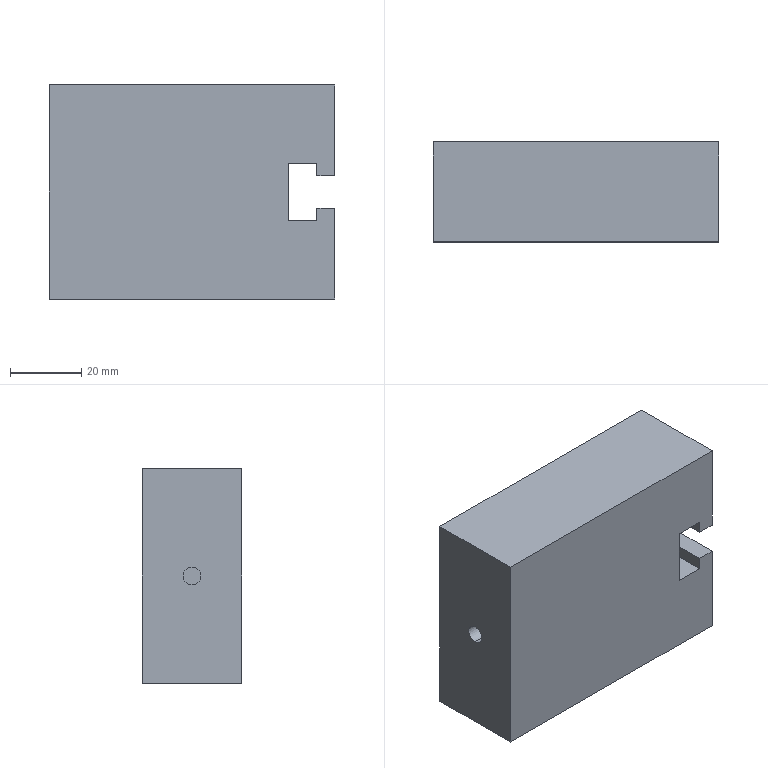Part | STEP file | 1 solid | 17 faces | box 80 x 28 x 60 mm | volume 129360 mm3 | plane 15 | cylinder 2 | commonest cylinder face diameters 5 x2
STEP:
#1=CARTESIAN_POINT('',(0.,0.,0.));
#2=DIRECTION('',(0.,0.,1.));
#3=DIRECTION('',(1.,0.,0.));
#4=AXIS2_PLACEMENT_3D('',#1,#2,#3);
#5=CARTESIAN_POINT('',(-30.,14.,2.5));
#6=VERTEX_POINT('',#5);
#7=CARTESIAN_POINT('',(-40.,14.,2.5));
#8=VERTEX_POINT('',#7);
#9=CARTESIAN_POINT('',(-30.,14.,2.5));
#10=DIRECTION('',(-1.,0.,0.));
#11=VECTOR('',#10,1.);
#12=LINE('',#9,#11);
#13=CARTESIAN_POINT('',(-30.,14.,0.));
#14=DIRECTION('',(-1.,0.,0.));
#15=DIRECTION('',(0.,0.,1.));
#16=AXIS2_PLACEMENT_3D('',#13,#14,#15);
#17=CYLINDRICAL_SURFACE('',#16,2.5);
#18=CARTESIAN_POINT('',(6.283,0.));
#19=DIRECTION('',(0.,1.));
#20=VECTOR('',#19,1.);
#21=LINE('',#18,#20);
#22=(GEOMETRIC_REPRESENTATION_CONTEXT(2)PARAMETRIC_REPRESENTATION_CONTEXT()REPRESENTATION_CONTEXT('',''));
#23=DEFINITIONAL_REPRESENTATION('',(#21),#22);
#24=PCURVE('',#17,#23);
#25=CARTESIAN_POINT('',(-30.,14.,0.));
#26=DIRECTION('',(-1.,0.,0.));
#27=DIRECTION('',(0.,0.,1.));
#28=AXIS2_PLACEMENT_3D('',#25,#26,#27);
#29=CYLINDRICAL_SURFACE('',#28,2.5);
#30=CARTESIAN_POINT('',(0.,0.));
#31=DIRECTION('',(0.,1.));
#32=VECTOR('',#31,1.);
#33=LINE('',#30,#32);
#34=(GEOMETRIC_REPRESENTATION_CONTEXT(2)PARAMETRIC_REPRESENTATION_CONTEXT()REPRESENTATION_CONTEXT('',''));
#35=DEFINITIONAL_REPRESENTATION('',(#33),#34);
#36=PCURVE('',#29,#35);
#37=SURFACE_CURVE('',#12,(#24,#36),.PCURVE_S1.);
#38=EDGE_CURVE('',#6,#8,#37,.T.);
#39=ORIENTED_EDGE('',*,*,#38,.T.);
#40=CARTESIAN_POINT('',(-40.,14.,-2.5));
#41=VERTEX_POINT('',#40);
#42=CARTESIAN_POINT('',(-40.,14.,0.));
#43=DIRECTION('',(-1.,0.,0.));
#44=DIRECTION('',(0.,0.,1.));
#45=AXIS2_PLACEMENT_3D('',#42,#43,#44);
#46=CIRCLE('',#45,2.5);
#47=CARTESIAN_POINT('',(0.,10.));
#48=DIRECTION('',(1.,0.));
#49=VECTOR('',#48,1.);
#50=LINE('',#47,#49);
#51=(GEOMETRIC_REPRESENTATION_CONTEXT(2)PARAMETRIC_REPRESENTATION_CONTEXT()REPRESENTATION_CONTEXT('',''));
#52=DEFINITIONAL_REPRESENTATION('',(#50),#51);
#53=PCURVE('',#17,#52);
#54=CARTESIAN_POINT('',(-40.,28.,30.));
#55=DIRECTION('',(1.,0.,0.));
#56=DIRECTION('',(0.,0.,-1.));
#57=AXIS2_PLACEMENT_3D('',#54,#55,#56);
#58=PLANE('',#57);
#59=CARTESIAN_POINT('',(27.5,-14.));
#60=CARTESIAN_POINT('',(27.5,-9.67));
#61=CARTESIAN_POINT('',(31.25,-11.835));
#62=CARTESIAN_POINT('',(35.,-14.));
#63=CARTESIAN_POINT('',(31.25,-16.165));
#64=CARTESIAN_POINT('',(27.5,-18.33));
#65=CARTESIAN_POINT('',(27.5,-14.));
#66=(BOUNDED_CURVE()B_SPLINE_CURVE(2,(#59,#60,#61,#62,#63,#64,#65),.UNSPECIFIED.,.T.,.F.)B_SPLINE_CURVE_WITH_KNOTS((1,2,2,2,2,1),(-2.094,0.,2.094,4.189,6.283,8.378),.UNSPECIFIED.)CURVE()GEOMETRIC_REPRESENTATION_ITEM()RATIONAL_B_SPLINE_CURVE((1.,0.5,1.,0.5,1.,0.5,1.))REPRESENTATION_ITEM(''));
#67=(GEOMETRIC_REPRESENTATION_CONTEXT(2)PARAMETRIC_REPRESENTATION_CONTEXT()REPRESENTATION_CONTEXT('',''));
#68=DEFINITIONAL_REPRESENTATION('',(#66),#67);
#69=PCURVE('',#58,#68);
#70=SURFACE_CURVE('',#46,(#53,#69),.PCURVE_S1.);
#71=EDGE_CURVE('',#41,#8,#70,.T.);
#72=ORIENTED_EDGE('',*,*,#71,.F.);
#73=CARTESIAN_POINT('',(-30.,14.,-2.5));
#74=VERTEX_POINT('',#73);
#75=CARTESIAN_POINT('',(-30.,14.,-2.5));
#76=DIRECTION('',(-1.,0.,0.));
#77=VECTOR('',#76,1.);
#78=LINE('',#75,#77);
#79=CARTESIAN_POINT('',(3.142,0.));
#80=DIRECTION('',(0.,1.));
#81=VECTOR('',#80,1.);
#82=LINE('',#79,#81);
#83=(GEOMETRIC_REPRESENTATION_CONTEXT(2)PARAMETRIC_REPRESENTATION_CONTEXT()REPRESENTATION_CONTEXT('',''));
#84=DEFINITIONAL_REPRESENTATION('',(#82),#83);
#85=PCURVE('',#17,#84);
#86=CARTESIAN_POINT('',(3.142,0.));
#87=DIRECTION('',(0.,1.));
#88=VECTOR('',#87,1.);
#89=LINE('',#86,#88);
#90=(GEOMETRIC_REPRESENTATION_CONTEXT(2)PARAMETRIC_REPRESENTATION_CONTEXT()REPRESENTATION_CONTEXT('',''));
#91=DEFINITIONAL_REPRESENTATION('',(#89),#90);
#92=PCURVE('',#29,#91);
#93=SURFACE_CURVE('',#78,(#85,#92),.PCURVE_S1.);
#94=EDGE_CURVE('',#74,#41,#93,.T.);
#95=ORIENTED_EDGE('',*,*,#94,.F.);
#96=CARTESIAN_POINT('',(-30.,14.,0.));
#97=DIRECTION('',(-1.,0.,0.));
#98=DIRECTION('',(0.,0.,1.));
#99=AXIS2_PLACEMENT_3D('',#96,#97,#98);
#100=CIRCLE('',#99,2.5);
#101=CARTESIAN_POINT('',(0.,0.));
#102=DIRECTION('',(1.,0.));
#103=VECTOR('',#102,1.);
#104=LINE('',#101,#103);
#105=(GEOMETRIC_REPRESENTATION_CONTEXT(2)PARAMETRIC_REPRESENTATION_CONTEXT()REPRESENTATION_CONTEXT('',''));
#106=DEFINITIONAL_REPRESENTATION('',(#104),#105);
#107=PCURVE('',#17,#106);
#108=CARTESIAN_POINT('',(-30.,14.,0.));
#109=DIRECTION('',(-1.,0.,0.));
#110=DIRECTION('',(0.,0.,1.));
#111=AXIS2_PLACEMENT_3D('',#108,#109,#110);
#112=PLANE('',#111);
#113=CARTESIAN_POINT('',(0.,0.));
#114=DIRECTION('',(1.,0.));
#115=AXIS2_PLACEMENT_2D('',#113,#114);
#116=CIRCLE('',#115,2.5);
#117=(GEOMETRIC_REPRESENTATION_CONTEXT(2)PARAMETRIC_REPRESENTATION_CONTEXT()REPRESENTATION_CONTEXT('',''));
#118=DEFINITIONAL_REPRESENTATION('',(#116),#117);
#119=PCURVE('',#112,#118);
#120=SURFACE_CURVE('',#100,(#107,#119),.PCURVE_S1.);
#121=EDGE_CURVE('',#74,#6,#120,.T.);
#122=ORIENTED_EDGE('',*,*,#121,.T.);
#123=EDGE_LOOP('',(#39,#72,#95,#122));
#124=FACE_BOUND('',#123,.F.);
#125=ADVANCED_FACE('',(#124),#17,.F.);
#126=CARTESIAN_POINT('',(40.,0.,30.));
#127=VERTEX_POINT('',#126);
#128=CARTESIAN_POINT('',(40.,0.,4.5));
#129=VERTEX_POINT('',#128);
#130=CARTESIAN_POINT('',(40.,0.,30.));
#131=DIRECTION('',(0.,0.,-1.));
#132=VECTOR('',#131,1.);
#133=LINE('',#130,#132);
#134=CARTESIAN_POINT('',(40.,28.,30.));
#135=DIRECTION('',(-1.,0.,0.));
#136=DIRECTION('',(0.,0.,1.));
#137=AXIS2_PLACEMENT_3D('',#134,#135,#136);
#138=PLANE('',#137);
#139=CARTESIAN_POINT('',(0.,-28.));
#140=DIRECTION('',(-1.,0.));
#141=VECTOR('',#140,1.);
#142=LINE('',#139,#141);
#143=(GEOMETRIC_REPRESENTATION_CONTEXT(2)PARAMETRIC_REPRESENTATION_CONTEXT()REPRESENTATION_CONTEXT('',''));
#144=DEFINITIONAL_REPRESENTATION('',(#142),#143);
#145=PCURVE('',#138,#144);
#146=CARTESIAN_POINT('',(0.,0.,0.));
#147=DIRECTION('',(0.,1.,0.));
#148=DIRECTION('',(0.,0.,1.));
#149=AXIS2_PLACEMENT_3D('',#146,#147,#148);
#150=PLANE('',#149);
#151=CARTESIAN_POINT('',(30.,40.));
#152=DIRECTION('',(-1.,0.));
#153=VECTOR('',#152,1.);
#154=LINE('',#151,#153);
#155=(GEOMETRIC_REPRESENTATION_CONTEXT(2)PARAMETRIC_REPRESENTATION_CONTEXT()REPRESENTATION_CONTEXT('',''));
#156=DEFINITIONAL_REPRESENTATION('',(#154),#155);
#157=PCURVE('',#150,#156);
#158=SURFACE_CURVE('',#133,(#145,#157),.PCURVE_S1.);
#159=EDGE_CURVE('',#127,#129,#158,.T.);
#160=ORIENTED_EDGE('',*,*,#159,.T.);
#161=CARTESIAN_POINT('',(40.,28.,4.5));
#162=VERTEX_POINT('',#161);
#163=CARTESIAN_POINT('',(40.,0.,4.5));
#164=DIRECTION('',(0.,1.,0.));
#165=VECTOR('',#164,1.);
#166=LINE('',#163,#165);
#167=CARTESIAN_POINT('',(-25.5,-28.));
#168=DIRECTION('',(0.,1.));
#169=VECTOR('',#168,1.);
#170=LINE('',#167,#169);
#171=(GEOMETRIC_REPRESENTATION_CONTEXT(2)PARAMETRIC_REPRESENTATION_CONTEXT()REPRESENTATION_CONTEXT('',''));
#172=DEFINITIONAL_REPRESENTATION('',(#170),#171);
#173=PCURVE('',#138,#172);
#174=CARTESIAN_POINT('',(40.,0.,4.5));
#175=DIRECTION('',(0.,0.,1.));
#176=DIRECTION('',(1.,0.,0.));
#177=AXIS2_PLACEMENT_3D('',#174,#175,#176);
#178=PLANE('',#177);
#179=CARTESIAN_POINT('',(0.,0.));
#180=DIRECTION('',(0.,1.));
#181=VECTOR('',#180,1.);
#182=LINE('',#179,#181);
#183=(GEOMETRIC_REPRESENTATION_CONTEXT(2)PARAMETRIC_REPRESENTATION_CONTEXT()REPRESENTATION_CONTEXT('',''));
#184=DEFINITIONAL_REPRESENTATION('',(#182),#183);
#185=PCURVE('',#178,#184);
#186=SURFACE_CURVE('',#166,(#173,#185),.PCURVE_S1.);
#187=EDGE_CURVE('',#129,#162,#186,.T.);
#188=ORIENTED_EDGE('',*,*,#187,.T.);
#189=CARTESIAN_POINT('',(40.,28.,30.));
#190=VERTEX_POINT('',#189);
#191=CARTESIAN_POINT('',(40.,28.,30.));
#192=DIRECTION('',(0.,0.,-1.));
#193=VECTOR('',#192,1.);
#194=LINE('',#191,#193);
#195=CARTESIAN_POINT('',(0.,0.));
#196=DIRECTION('',(-1.,0.));
#197=VECTOR('',#196,1.);
#198=LINE('',#195,#197);
#199=(GEOMETRIC_REPRESENTATION_CONTEXT(2)PARAMETRIC_REPRESENTATION_CONTEXT()REPRESENTATION_CONTEXT('',''));
#200=DEFINITIONAL_REPRESENTATION('',(#198),#199);
#201=PCURVE('',#138,#200);
#202=CARTESIAN_POINT('',(0.,28.,0.));
#203=DIRECTION('',(0.,1.,0.));
#204=DIRECTION('',(0.,0.,1.));
#205=AXIS2_PLACEMENT_3D('',#202,#203,#204);
#206=PLANE('',#205);
#207=CARTESIAN_POINT('',(30.,40.));
#208=DIRECTION('',(-1.,0.));
#209=VECTOR('',#208,1.);
#210=LINE('',#207,#209);
#211=(GEOMETRIC_REPRESENTATION_CONTEXT(2)PARAMETRIC_REPRESENTATION_CONTEXT()REPRESENTATION_CONTEXT('',''));
#212=DEFINITIONAL_REPRESENTATION('',(#210),#211);
#213=PCURVE('',#206,#212);
#214=SURFACE_CURVE('',#194,(#201,#213),.PCURVE_S1.);
#215=EDGE_CURVE('',#190,#162,#214,.T.);
#216=ORIENTED_EDGE('',*,*,#215,.F.);
#217=CARTESIAN_POINT('',(40.,28.,30.));
#218=DIRECTION('',(0.,-1.,0.));
#219=VECTOR('',#218,1.);
#220=LINE('',#217,#219);
#221=CARTESIAN_POINT('',(0.,0.));
#222=DIRECTION('',(0.,-1.));
#223=VECTOR('',#222,1.);
#224=LINE('',#221,#223);
#225=(GEOMETRIC_REPRESENTATION_CONTEXT(2)PARAMETRIC_REPRESENTATION_CONTEXT()REPRESENTATION_CONTEXT('',''));
#226=DEFINITIONAL_REPRESENTATION('',(#224),#225);
#227=PCURVE('',#138,#226);
#228=CARTESIAN_POINT('',(40.,28.,30.));
#229=DIRECTION('',(0.,0.,-1.));
#230=DIRECTION('',(-1.,0.,0.));
#231=AXIS2_PLACEMENT_3D('',#228,#229,#230);
#232=PLANE('',#231);
#233=CARTESIAN_POINT('',(0.,0.));
#234=DIRECTION('',(0.,-1.));
#235=VECTOR('',#234,1.);
#236=LINE('',#233,#235);
#237=(GEOMETRIC_REPRESENTATION_CONTEXT(2)PARAMETRIC_REPRESENTATION_CONTEXT()REPRESENTATION_CONTEXT('',''));
#238=DEFINITIONAL_REPRESENTATION('',(#236),#237);
#239=PCURVE('',#232,#238);
#240=SURFACE_CURVE('',#220,(#227,#239),.PCURVE_S1.);
#241=EDGE_CURVE('',#190,#127,#240,.T.);
#242=ORIENTED_EDGE('',*,*,#241,.T.);
#243=EDGE_LOOP('',(#160,#188,#216,#242));
#244=FACE_BOUND('',#243,.T.);
#245=ADVANCED_FACE('',(#244),#138,.F.);
#246=CARTESIAN_POINT('',(-40.,14.,0.));
#247=DIRECTION('',(-1.,0.,0.));
#248=DIRECTION('',(0.,0.,1.));
#249=AXIS2_PLACEMENT_3D('',#246,#247,#248);
#250=CIRCLE('',#249,2.5);
#251=CARTESIAN_POINT('',(27.5,-14.));
#252=CARTESIAN_POINT('',(27.5,-9.67));
#253=CARTESIAN_POINT('',(31.25,-11.835));
#254=CARTESIAN_POINT('',(35.,-14.));
#255=CARTESIAN_POINT('',(31.25,-16.165));
#256=CARTESIAN_POINT('',(27.5,-18.33));
#257=CARTESIAN_POINT('',(27.5,-14.));
#258=(BOUNDED_CURVE()B_SPLINE_CURVE(2,(#251,#252,#253,#254,#255,#256,#257),.UNSPECIFIED.,.T.,.F.)B_SPLINE_CURVE_WITH_KNOTS((1,2,2,2,2,1),(-2.094,0.,2.094,4.189,6.283,8.378),.UNSPECIFIED.)CURVE()GEOMETRIC_REPRESENTATION_ITEM()RATIONAL_B_SPLINE_CURVE((1.,0.5,1.,0.5,1.,0.5,1.))REPRESENTATION_ITEM(''));
#259=(GEOMETRIC_REPRESENTATION_CONTEXT(2)PARAMETRIC_REPRESENTATION_CONTEXT()REPRESENTATION_CONTEXT('',''));
#260=DEFINITIONAL_REPRESENTATION('',(#258),#259);
#261=PCURVE('',#58,#260);
#262=CARTESIAN_POINT('',(0.,10.));
#263=DIRECTION('',(1.,0.));
#264=VECTOR('',#263,1.);
#265=LINE('',#262,#264);
#266=(GEOMETRIC_REPRESENTATION_CONTEXT(2)PARAMETRIC_REPRESENTATION_CONTEXT()REPRESENTATION_CONTEXT('',''));
#267=DEFINITIONAL_REPRESENTATION('',(#265),#266);
#268=PCURVE('',#29,#267);
#269=SURFACE_CURVE('',#250,(#261,#268),.PCURVE_S1.);
#270=EDGE_CURVE('',#8,#41,#269,.T.);
#271=ORIENTED_EDGE('',*,*,#270,.F.);
#272=ORIENTED_EDGE('',*,*,#71,.F.);
#273=EDGE_LOOP('',(#271,#272));
#274=FACE_BOUND('',#273,.T.);
#275=CARTESIAN_POINT('',(-40.,0.,-30.));
#276=VERTEX_POINT('',#275);
#277=CARTESIAN_POINT('',(-40.,0.,30.));
#278=VERTEX_POINT('',#277);
#279=CARTESIAN_POINT('',(-40.,0.,30.));
#280=DIRECTION('',(0.,0.,1.));
#281=VECTOR('',#280,1.);
#282=LINE('',#279,#281);
#283=CARTESIAN_POINT('',(0.,-28.));
#284=DIRECTION('',(-1.,0.));
#285=VECTOR('',#284,1.);
#286=LINE('',#283,#285);
#287=(GEOMETRIC_REPRESENTATION_CONTEXT(2)PARAMETRIC_REPRESENTATION_CONTEXT()REPRESENTATION_CONTEXT('',''));
#288=DEFINITIONAL_REPRESENTATION('',(#286),#287);
#289=PCURVE('',#58,#288);
#290=CARTESIAN_POINT('',(30.,-40.));
#291=DIRECTION('',(1.,0.));
#292=VECTOR('',#291,1.);
#293=LINE('',#290,#292);
#294=(GEOMETRIC_REPRESENTATION_CONTEXT(2)PARAMETRIC_REPRESENTATION_CONTEXT()REPRESENTATION_CONTEXT('',''));
#295=DEFINITIONAL_REPRESENTATION('',(#293),#294);
#296=PCURVE('',#150,#295);
#297=SURFACE_CURVE('',#282,(#289,#296),.PCURVE_S1.);
#298=EDGE_CURVE('',#276,#278,#297,.T.);
#299=ORIENTED_EDGE('',*,*,#298,.T.);
#300=CARTESIAN_POINT('',(-40.,28.,30.));
#301=VERTEX_POINT('',#300);
#302=CARTESIAN_POINT('',(-40.,28.,30.));
#303=DIRECTION('',(0.,-1.,0.));
#304=VECTOR('',#303,1.);
#305=LINE('',#302,#304);
#306=CARTESIAN_POINT('',(0.,0.));
#307=DIRECTION('',(0.,-1.));
#308=VECTOR('',#307,1.);
#309=LINE('',#306,#308);
#310=(GEOMETRIC_REPRESENTATION_CONTEXT(2)PARAMETRIC_REPRESENTATION_CONTEXT()REPRESENTATION_CONTEXT('',''));
#311=DEFINITIONAL_REPRESENTATION('',(#309),#310);
#312=PCURVE('',#58,#311);
#313=CARTESIAN_POINT('',(80.,0.));
#314=DIRECTION('',(0.,-1.));
#315=VECTOR('',#314,1.);
#316=LINE('',#313,#315);
#317=(GEOMETRIC_REPRESENTATION_CONTEXT(2)PARAMETRIC_REPRESENTATION_CONTEXT()REPRESENTATION_CONTEXT('',''));
#318=DEFINITIONAL_REPRESENTATION('',(#316),#317);
#319=PCURVE('',#232,#318);
#320=SURFACE_CURVE('',#305,(#312,#319),.PCURVE_S1.);
#321=EDGE_CURVE('',#301,#278,#320,.T.);
#322=ORIENTED_EDGE('',*,*,#321,.F.);
#323=CARTESIAN_POINT('',(-40.,28.,-30.));
#324=VERTEX_POINT('',#323);
#325=CARTESIAN_POINT('',(-40.,28.,30.));
#326=DIRECTION('',(0.,0.,1.));
#327=VECTOR('',#326,1.);
#328=LINE('',#325,#327);
#329=CARTESIAN_POINT('',(0.,0.));
#330=DIRECTION('',(-1.,0.));
#331=VECTOR('',#330,1.);
#332=LINE('',#329,#331);
#333=(GEOMETRIC_REPRESENTATION_CONTEXT(2)PARAMETRIC_REPRESENTATION_CONTEXT()REPRESENTATION_CONTEXT('',''));
#334=DEFINITIONAL_REPRESENTATION('',(#332),#333);
#335=PCURVE('',#58,#334);
#336=CARTESIAN_POINT('',(30.,-40.));
#337=DIRECTION('',(1.,0.));
#338=VECTOR('',#337,1.);
#339=LINE('',#336,#338);
#340=(GEOMETRIC_REPRESENTATION_CONTEXT(2)PARAMETRIC_REPRESENTATION_CONTEXT()REPRESENTATION_CONTEXT('',''));
#341=DEFINITIONAL_REPRESENTATION('',(#339),#340);
#342=PCURVE('',#206,#341);
#343=SURFACE_CURVE('',#328,(#335,#342),.PCURVE_S1.);
#344=EDGE_CURVE('',#324,#301,#343,.T.);
#345=ORIENTED_EDGE('',*,*,#344,.F.);
#346=CARTESIAN_POINT('',(-40.,28.,-30.));
#347=DIRECTION('',(0.,-1.,0.));
#348=VECTOR('',#347,1.);
#349=LINE('',#346,#348);
#350=CARTESIAN_POINT('',(60.,0.));
#351=DIRECTION('',(0.,-1.));
#352=VECTOR('',#351,1.);
#353=LINE('',#350,#352);
#354=(GEOMETRIC_REPRESENTATION_CONTEXT(2)PARAMETRIC_REPRESENTATION_CONTEXT()REPRESENTATION_CONTEXT('',''));
#355=DEFINITIONAL_REPRESENTATION('',(#353),#354);
#356=PCURVE('',#58,#355);
#357=CARTESIAN_POINT('',(40.,28.,-30.));
#358=DIRECTION('',(0.,0.,1.));
#359=DIRECTION('',(1.,0.,0.));
#360=AXIS2_PLACEMENT_3D('',#357,#358,#359);
#361=PLANE('',#360);
#362=CARTESIAN_POINT('',(-80.,0.));
#363=DIRECTION('',(0.,-1.));
#364=VECTOR('',#363,1.);
#365=LINE('',#362,#364);
#366=(GEOMETRIC_REPRESENTATION_CONTEXT(2)PARAMETRIC_REPRESENTATION_CONTEXT()REPRESENTATION_CONTEXT('',''));
#367=DEFINITIONAL_REPRESENTATION('',(#365),#366);
#368=PCURVE('',#361,#367);
#369=SURFACE_CURVE('',#349,(#356,#368),.PCURVE_S1.);
#370=EDGE_CURVE('',#324,#276,#369,.T.);
#371=ORIENTED_EDGE('',*,*,#370,.T.);
#372=EDGE_LOOP('',(#299,#322,#345,#371));
#373=FACE_BOUND('',#372,.T.);
#374=ADVANCED_FACE('',(#274,#373),#58,.F.);
#375=CARTESIAN_POINT('',(40.,0.,30.));
#376=DIRECTION('',(1.,0.,0.));
#377=VECTOR('',#376,1.);
#378=LINE('',#375,#377);
#379=CARTESIAN_POINT('',(0.,-28.));
#380=DIRECTION('',(-1.,0.));
#381=VECTOR('',#380,1.);
#382=LINE('',#379,#381);
#383=(GEOMETRIC_REPRESENTATION_CONTEXT(2)PARAMETRIC_REPRESENTATION_CONTEXT()REPRESENTATION_CONTEXT('',''));
#384=DEFINITIONAL_REPRESENTATION('',(#382),#383);
#385=PCURVE('',#232,#384);
#386=CARTESIAN_POINT('',(30.,40.));
#387=DIRECTION('',(0.,1.));
#388=VECTOR('',#387,1.);
#389=LINE('',#386,#388);
#390=(GEOMETRIC_REPRESENTATION_CONTEXT(2)PARAMETRIC_REPRESENTATION_CONTEXT()REPRESENTATION_CONTEXT('',''));
#391=DEFINITIONAL_REPRESENTATION('',(#389),#390);
#392=PCURVE('',#150,#391);
#393=SURFACE_CURVE('',#378,(#385,#392),.PCURVE_S1.);
#394=EDGE_CURVE('',#278,#127,#393,.T.);
#395=ORIENTED_EDGE('',*,*,#394,.T.);
#396=ORIENTED_EDGE('',*,*,#241,.F.);
#397=CARTESIAN_POINT('',(40.,28.,30.));
#398=DIRECTION('',(1.,0.,0.));
#399=VECTOR('',#398,1.);
#400=LINE('',#397,#399);
#401=CARTESIAN_POINT('',(0.,0.));
#402=DIRECTION('',(-1.,0.));
#403=VECTOR('',#402,1.);
#404=LINE('',#401,#403);
#405=(GEOMETRIC_REPRESENTATION_CONTEXT(2)PARAMETRIC_REPRESENTATION_CONTEXT()REPRESENTATION_CONTEXT('',''));
#406=DEFINITIONAL_REPRESENTATION('',(#404),#405);
#407=PCURVE('',#232,#406);
#408=CARTESIAN_POINT('',(30.,40.));
#409=DIRECTION('',(0.,1.));
#410=VECTOR('',#409,1.);
#411=LINE('',#408,#410);
#412=(GEOMETRIC_REPRESENTATION_CONTEXT(2)PARAMETRIC_REPRESENTATION_CONTEXT()REPRESENTATION_CONTEXT('',''));
#413=DEFINITIONAL_REPRESENTATION('',(#411),#412);
#414=PCURVE('',#206,#413);
#415=SURFACE_CURVE('',#400,(#407,#414),.PCURVE_S1.);
#416=EDGE_CURVE('',#301,#190,#415,.T.);
#417=ORIENTED_EDGE('',*,*,#416,.F.);
#418=ORIENTED_EDGE('',*,*,#321,.T.);
#419=EDGE_LOOP('',(#395,#396,#417,#418));
#420=FACE_BOUND('',#419,.T.);
#421=ADVANCED_FACE('',(#420),#232,.F.);
#422=CARTESIAN_POINT('',(40.,28.,-4.5));
#423=VERTEX_POINT('',#422);
#424=CARTESIAN_POINT('',(40.,28.,-30.));
#425=VERTEX_POINT('',#424);
#426=CARTESIAN_POINT('',(40.,28.,30.));
#427=DIRECTION('',(0.,0.,-1.));
#428=VECTOR('',#427,1.);
#429=LINE('',#426,#428);
#430=CARTESIAN_POINT('',(40.,28.,30.));
#431=DIRECTION('',(-1.,0.,0.));
#432=DIRECTION('',(0.,0.,1.));
#433=AXIS2_PLACEMENT_3D('',#430,#431,#432);
#434=PLANE('',#433);
#435=CARTESIAN_POINT('',(0.,0.));
#436=DIRECTION('',(-1.,0.));
#437=VECTOR('',#436,1.);
#438=LINE('',#435,#437);
#439=(GEOMETRIC_REPRESENTATION_CONTEXT(2)PARAMETRIC_REPRESENTATION_CONTEXT()REPRESENTATION_CONTEXT('',''));
#440=DEFINITIONAL_REPRESENTATION('',(#438),#439);
#441=PCURVE('',#434,#440);
#442=CARTESIAN_POINT('',(30.,40.));
#443=DIRECTION('',(-1.,0.));
#444=VECTOR('',#443,1.);
#445=LINE('',#442,#444);
#446=(GEOMETRIC_REPRESENTATION_CONTEXT(2)PARAMETRIC_REPRESENTATION_CONTEXT()REPRESENTATION_CONTEXT('',''));
#447=DEFINITIONAL_REPRESENTATION('',(#445),#446);
#448=PCURVE('',#206,#447);
#449=SURFACE_CURVE('',#429,(#441,#448),.PCURVE_S1.);
#450=EDGE_CURVE('',#423,#425,#449,.T.);
#451=ORIENTED_EDGE('',*,*,#450,.F.);
#452=CARTESIAN_POINT('',(40.,0.,-4.5));
#453=VERTEX_POINT('',#452);
#454=CARTESIAN_POINT('',(40.,0.,-4.5));
#455=DIRECTION('',(0.,1.,0.));
#456=VECTOR('',#455,1.);
#457=LINE('',#454,#456);
#458=CARTESIAN_POINT('',(-34.5,-28.));
#459=DIRECTION('',(0.,1.));
#460=VECTOR('',#459,1.);
#461=LINE('',#458,#460);
#462=(GEOMETRIC_REPRESENTATION_CONTEXT(2)PARAMETRIC_REPRESENTATION_CONTEXT()REPRESENTATION_CONTEXT('',''));
#463=DEFINITIONAL_REPRESENTATION('',(#461),#462);
#464=PCURVE('',#434,#463);
#465=CARTESIAN_POINT('',(40.,0.,-4.5));
#466=DIRECTION('',(0.,0.,-1.));
#467=DIRECTION('',(-1.,0.,0.));
#468=AXIS2_PLACEMENT_3D('',#465,#466,#467);
#469=PLANE('',#468);
#470=CARTESIAN_POINT('',(0.,0.));
#471=DIRECTION('',(0.,1.));
#472=VECTOR('',#471,1.);
#473=LINE('',#470,#472);
#474=(GEOMETRIC_REPRESENTATION_CONTEXT(2)PARAMETRIC_REPRESENTATION_CONTEXT()REPRESENTATION_CONTEXT('',''));
#475=DEFINITIONAL_REPRESENTATION('',(#473),#474);
#476=PCURVE('',#469,#475);
#477=SURFACE_CURVE('',#457,(#464,#476),.PCURVE_S1.);
#478=EDGE_CURVE('',#453,#423,#477,.T.);
#479=ORIENTED_EDGE('',*,*,#478,.F.);
#480=CARTESIAN_POINT('',(40.,0.,-30.));
#481=VERTEX_POINT('',#480);
#482=CARTESIAN_POINT('',(40.,0.,30.));
#483=DIRECTION('',(0.,0.,-1.));
#484=VECTOR('',#483,1.);
#485=LINE('',#482,#484);
#486=CARTESIAN_POINT('',(0.,-28.));
#487=DIRECTION('',(-1.,0.));
#488=VECTOR('',#487,1.);
#489=LINE('',#486,#488);
#490=(GEOMETRIC_REPRESENTATION_CONTEXT(2)PARAMETRIC_REPRESENTATION_CONTEXT()REPRESENTATION_CONTEXT('',''));
#491=DEFINITIONAL_REPRESENTATION('',(#489),#490);
#492=PCURVE('',#434,#491);
#493=CARTESIAN_POINT('',(30.,40.));
#494=DIRECTION('',(-1.,0.));
#495=VECTOR('',#494,1.);
#496=LINE('',#493,#495);
#497=(GEOMETRIC_REPRESENTATION_CONTEXT(2)PARAMETRIC_REPRESENTATION_CONTEXT()REPRESENTATION_CONTEXT('',''));
#498=DEFINITIONAL_REPRESENTATION('',(#496),#497);
#499=PCURVE('',#150,#498);
#500=SURFACE_CURVE('',#485,(#492,#499),.PCURVE_S1.);
#501=EDGE_CURVE('',#453,#481,#500,.T.);
#502=ORIENTED_EDGE('',*,*,#501,.T.);
#503=CARTESIAN_POINT('',(40.,28.,-30.));
#504=DIRECTION('',(0.,-1.,0.));
#505=VECTOR('',#504,1.);
#506=LINE('',#503,#505);
#507=CARTESIAN_POINT('',(-60.,0.));
#508=DIRECTION('',(0.,-1.));
#509=VECTOR('',#508,1.);
#510=LINE('',#507,#509);
#511=(GEOMETRIC_REPRESENTATION_CONTEXT(2)PARAMETRIC_REPRESENTATION_CONTEXT()REPRESENTATION_CONTEXT('',''));
#512=DEFINITIONAL_REPRESENTATION('',(#510),#511);
#513=PCURVE('',#434,#512);
#514=CARTESIAN_POINT('',(0.,0.));
#515=DIRECTION('',(0.,-1.));
#516=VECTOR('',#515,1.);
#517=LINE('',#514,#516);
#518=(GEOMETRIC_REPRESENTATION_CONTEXT(2)PARAMETRIC_REPRESENTATION_CONTEXT()REPRESENTATION_CONTEXT('',''));
#519=DEFINITIONAL_REPRESENTATION('',(#517),#518);
#520=PCURVE('',#361,#519);
#521=SURFACE_CURVE('',#506,(#513,#520),.PCURVE_S1.);
#522=EDGE_CURVE('',#425,#481,#521,.T.);
#523=ORIENTED_EDGE('',*,*,#522,.F.);
#524=EDGE_LOOP('',(#451,#479,#502,#523));
#525=FACE_BOUND('',#524,.T.);
#526=ADVANCED_FACE('',(#525),#434,.F.);
#527=CARTESIAN_POINT('',(40.,0.,-30.));
#528=DIRECTION('',(-1.,0.,0.));
#529=VECTOR('',#528,1.);
#530=LINE('',#527,#529);
#531=CARTESIAN_POINT('',(0.,-28.));
#532=DIRECTION('',(-1.,0.));
#533=VECTOR('',#532,1.);
#534=LINE('',#531,#533);
#535=(GEOMETRIC_REPRESENTATION_CONTEXT(2)PARAMETRIC_REPRESENTATION_CONTEXT()REPRESENTATION_CONTEXT('',''));
#536=DEFINITIONAL_REPRESENTATION('',(#534),#535);
#537=PCURVE('',#361,#536);
#538=CARTESIAN_POINT('',(-30.,40.));
#539=DIRECTION('',(0.,-1.));
#540=VECTOR('',#539,1.);
#541=LINE('',#538,#540);
#542=(GEOMETRIC_REPRESENTATION_CONTEXT(2)PARAMETRIC_REPRESENTATION_CONTEXT()REPRESENTATION_CONTEXT('',''));
#543=DEFINITIONAL_REPRESENTATION('',(#541),#542);
#544=PCURVE('',#150,#543);
#545=SURFACE_CURVE('',#530,(#537,#544),.PCURVE_S1.);
#546=EDGE_CURVE('',#481,#276,#545,.T.);
#547=ORIENTED_EDGE('',*,*,#546,.T.);
#548=ORIENTED_EDGE('',*,*,#370,.F.);
#549=CARTESIAN_POINT('',(40.,28.,-30.));
#550=DIRECTION('',(-1.,0.,0.));
#551=VECTOR('',#550,1.);
#552=LINE('',#549,#551);
#553=CARTESIAN_POINT('',(0.,0.));
#554=DIRECTION('',(-1.,0.));
#555=VECTOR('',#554,1.);
#556=LINE('',#553,#555);
#557=(GEOMETRIC_REPRESENTATION_CONTEXT(2)PARAMETRIC_REPRESENTATION_CONTEXT()REPRESENTATION_CONTEXT('',''));
#558=DEFINITIONAL_REPRESENTATION('',(#556),#557);
#559=PCURVE('',#361,#558);
#560=CARTESIAN_POINT('',(-30.,40.));
#561=DIRECTION('',(0.,-1.));
#562=VECTOR('',#561,1.);
#563=LINE('',#560,#562);
#564=(GEOMETRIC_REPRESENTATION_CONTEXT(2)PARAMETRIC_REPRESENTATION_CONTEXT()REPRESENTATION_CONTEXT('',''));
#565=DEFINITIONAL_REPRESENTATION('',(#563),#564);
#566=PCURVE('',#206,#565);
#567=SURFACE_CURVE('',#552,(#559,#566),.PCURVE_S1.);
#568=EDGE_CURVE('',#425,#324,#567,.T.);
#569=ORIENTED_EDGE('',*,*,#568,.F.);
#570=ORIENTED_EDGE('',*,*,#522,.T.);
#571=EDGE_LOOP('',(#547,#548,#569,#570));
#572=FACE_BOUND('',#571,.T.);
#573=ADVANCED_FACE('',(#572),#361,.F.);
#574=CARTESIAN_POINT('',(35.,28.,4.5));
#575=VERTEX_POINT('',#574);
#576=CARTESIAN_POINT('',(40.,28.,4.5));
#577=DIRECTION('',(1.,0.,0.));
#578=VECTOR('',#577,1.);
#579=LINE('',#576,#578);
#580=CARTESIAN_POINT('',(4.5,40.));
#581=DIRECTION('',(0.,1.));
#582=VECTOR('',#581,1.);
#583=LINE('',#580,#582);
#584=(GEOMETRIC_REPRESENTATION_CONTEXT(2)PARAMETRIC_REPRESENTATION_CONTEXT()REPRESENTATION_CONTEXT('',''));
#585=DEFINITIONAL_REPRESENTATION('',(#583),#584);
#586=PCURVE('',#206,#585);
#587=CARTESIAN_POINT('',(0.,28.));
#588=DIRECTION('',(1.,0.));
#589=VECTOR('',#588,1.);
#590=LINE('',#587,#589);
#591=(GEOMETRIC_REPRESENTATION_CONTEXT(2)PARAMETRIC_REPRESENTATION_CONTEXT()REPRESENTATION_CONTEXT('',''));
#592=DEFINITIONAL_REPRESENTATION('',(#590),#591);
#593=PCURVE('',#178,#592);
#594=SURFACE_CURVE('',#579,(#586,#593),.PCURVE_S1.);
#595=EDGE_CURVE('',#575,#162,#594,.T.);
#596=ORIENTED_EDGE('',*,*,#595,.F.);
#597=CARTESIAN_POINT('',(35.,28.,8.));
#598=VERTEX_POINT('',#597);
#599=CARTESIAN_POINT('',(35.,28.,4.5));
#600=DIRECTION('',(0.,0.,-1.));
#601=VECTOR('',#600,1.);
#602=LINE('',#599,#601);
#603=CARTESIAN_POINT('',(4.5,35.));
#604=DIRECTION('',(-1.,0.));
#605=VECTOR('',#604,1.);
#606=LINE('',#603,#605);
#607=(GEOMETRIC_REPRESENTATION_CONTEXT(2)PARAMETRIC_REPRESENTATION_CONTEXT()REPRESENTATION_CONTEXT('',''));
#608=DEFINITIONAL_REPRESENTATION('',(#606),#607);
#609=PCURVE('',#206,#608);
#610=CARTESIAN_POINT('',(35.,0.,4.5));
#611=DIRECTION('',(1.,0.,0.));
#612=DIRECTION('',(0.,0.,-1.));
#613=AXIS2_PLACEMENT_3D('',#610,#611,#612);
#614=PLANE('',#613);
#615=CARTESIAN_POINT('',(0.,28.));
#616=DIRECTION('',(1.,0.));
#617=VECTOR('',#616,1.);
#618=LINE('',#615,#617);
#619=(GEOMETRIC_REPRESENTATION_CONTEXT(2)PARAMETRIC_REPRESENTATION_CONTEXT()REPRESENTATION_CONTEXT('',''));
#620=DEFINITIONAL_REPRESENTATION('',(#618),#619);
#621=PCURVE('',#614,#620);
#622=SURFACE_CURVE('',#602,(#609,#621),.PCURVE_S1.);
#623=EDGE_CURVE('',#598,#575,#622,.T.);
#624=ORIENTED_EDGE('',*,*,#623,.F.);
#625=CARTESIAN_POINT('',(27.,28.,8.));
#626=VERTEX_POINT('',#625);
#627=CARTESIAN_POINT('',(35.,28.,8.));
#628=DIRECTION('',(1.,0.,0.));
#629=VECTOR('',#628,1.);
#630=LINE('',#627,#629);
#631=CARTESIAN_POINT('',(8.,35.));
#632=DIRECTION('',(0.,1.));
#633=VECTOR('',#632,1.);
#634=LINE('',#631,#633);
#635=(GEOMETRIC_REPRESENTATION_CONTEXT(2)PARAMETRIC_REPRESENTATION_CONTEXT()REPRESENTATION_CONTEXT('',''));
#636=DEFINITIONAL_REPRESENTATION('',(#634),#635);
#637=PCURVE('',#206,#636);
#638=CARTESIAN_POINT('',(35.,0.,8.));
#639=DIRECTION('',(0.,0.,1.));
#640=DIRECTION('',(1.,0.,0.));
#641=AXIS2_PLACEMENT_3D('',#638,#639,#640);
#642=PLANE('',#641);
#643=CARTESIAN_POINT('',(0.,28.));
#644=DIRECTION('',(1.,0.));
#645=VECTOR('',#644,1.);
#646=LINE('',#643,#645);
#647=(GEOMETRIC_REPRESENTATION_CONTEXT(2)PARAMETRIC_REPRESENTATION_CONTEXT()REPRESENTATION_CONTEXT('',''));
#648=DEFINITIONAL_REPRESENTATION('',(#646),#647);
#649=PCURVE('',#642,#648);
#650=SURFACE_CURVE('',#630,(#637,#649),.PCURVE_S1.);
#651=EDGE_CURVE('',#626,#598,#650,.T.);
#652=ORIENTED_EDGE('',*,*,#651,.F.);
#653=CARTESIAN_POINT('',(27.,28.,-8.));
#654=VERTEX_POINT('',#653);
#655=CARTESIAN_POINT('',(27.,28.,-8.));
#656=DIRECTION('',(0.,0.,1.));
#657=VECTOR('',#656,1.);
#658=LINE('',#655,#657);
#659=CARTESIAN_POINT('',(-8.,27.));
#660=DIRECTION('',(1.,0.));
#661=VECTOR('',#660,1.);
#662=LINE('',#659,#661);
#663=(GEOMETRIC_REPRESENTATION_CONTEXT(2)PARAMETRIC_REPRESENTATION_CONTEXT()REPRESENTATION_CONTEXT('',''));
#664=DEFINITIONAL_REPRESENTATION('',(#662),#663);
#665=PCURVE('',#206,#664);
#666=CARTESIAN_POINT('',(27.,0.,-8.));
#667=DIRECTION('',(-1.,0.,0.));
#668=DIRECTION('',(0.,0.,1.));
#669=AXIS2_PLACEMENT_3D('',#666,#667,#668);
#670=PLANE('',#669);
#671=CARTESIAN_POINT('',(0.,28.));
#672=DIRECTION('',(1.,0.));
#673=VECTOR('',#672,1.);
#674=LINE('',#671,#673);
#675=(GEOMETRIC_REPRESENTATION_CONTEXT(2)PARAMETRIC_REPRESENTATION_CONTEXT()REPRESENTATION_CONTEXT('',''));
#676=DEFINITIONAL_REPRESENTATION('',(#674),#675);
#677=PCURVE('',#670,#676);
#678=SURFACE_CURVE('',#658,(#665,#677),.PCURVE_S1.);
#679=EDGE_CURVE('',#654,#626,#678,.T.);
#680=ORIENTED_EDGE('',*,*,#679,.F.);
#681=CARTESIAN_POINT('',(35.,28.,-8.));
#682=VERTEX_POINT('',#681);
#683=CARTESIAN_POINT('',(35.,28.,-8.));
#684=DIRECTION('',(-1.,0.,0.));
#685=VECTOR('',#684,1.);
#686=LINE('',#683,#685);
#687=CARTESIAN_POINT('',(-8.,35.));
#688=DIRECTION('',(0.,-1.));
#689=VECTOR('',#688,1.);
#690=LINE('',#687,#689);
#691=(GEOMETRIC_REPRESENTATION_CONTEXT(2)PARAMETRIC_REPRESENTATION_CONTEXT()REPRESENTATION_CONTEXT('',''));
#692=DEFINITIONAL_REPRESENTATION('',(#690),#691);
#693=PCURVE('',#206,#692);
#694=CARTESIAN_POINT('',(35.,0.,-8.));
#695=DIRECTION('',(0.,0.,-1.));
#696=DIRECTION('',(-1.,0.,0.));
#697=AXIS2_PLACEMENT_3D('',#694,#695,#696);
#698=PLANE('',#697);
#699=CARTESIAN_POINT('',(0.,28.));
#700=DIRECTION('',(1.,0.));
#701=VECTOR('',#700,1.);
#702=LINE('',#699,#701);
#703=(GEOMETRIC_REPRESENTATION_CONTEXT(2)PARAMETRIC_REPRESENTATION_CONTEXT()REPRESENTATION_CONTEXT('',''));
#704=DEFINITIONAL_REPRESENTATION('',(#702),#703);
#705=PCURVE('',#698,#704);
#706=SURFACE_CURVE('',#686,(#693,#705),.PCURVE_S1.);
#707=EDGE_CURVE('',#682,#654,#706,.T.);
#708=ORIENTED_EDGE('',*,*,#707,.F.);
#709=CARTESIAN_POINT('',(35.,28.,-4.5));
#710=VERTEX_POINT('',#709);
#711=CARTESIAN_POINT('',(35.,28.,-4.5));
#712=DIRECTION('',(0.,0.,-1.));
#713=VECTOR('',#712,1.);
#714=LINE('',#711,#713);
#715=CARTESIAN_POINT('',(-4.5,35.));
#716=DIRECTION('',(-1.,0.));
#717=VECTOR('',#716,1.);
#718=LINE('',#715,#717);
#719=(GEOMETRIC_REPRESENTATION_CONTEXT(2)PARAMETRIC_REPRESENTATION_CONTEXT()REPRESENTATION_CONTEXT('',''));
#720=DEFINITIONAL_REPRESENTATION('',(#718),#719);
#721=PCURVE('',#206,#720);
#722=CARTESIAN_POINT('',(35.,0.,-4.5));
#723=DIRECTION('',(1.,0.,0.));
#724=DIRECTION('',(0.,0.,-1.));
#725=AXIS2_PLACEMENT_3D('',#722,#723,#724);
#726=PLANE('',#725);
#727=CARTESIAN_POINT('',(0.,28.));
#728=DIRECTION('',(1.,0.));
#729=VECTOR('',#728,1.);
#730=LINE('',#727,#729);
#731=(GEOMETRIC_REPRESENTATION_CONTEXT(2)PARAMETRIC_REPRESENTATION_CONTEXT()REPRESENTATION_CONTEXT('',''));
#732=DEFINITIONAL_REPRESENTATION('',(#730),#731);
#733=PCURVE('',#726,#732);
#734=SURFACE_CURVE('',#714,(#721,#733),.PCURVE_S1.);
#735=EDGE_CURVE('',#710,#682,#734,.T.);
#736=ORIENTED_EDGE('',*,*,#735,.F.);
#737=CARTESIAN_POINT('',(40.,28.,-4.5));
#738=DIRECTION('',(-1.,0.,0.));
#739=VECTOR('',#738,1.);
#740=LINE('',#737,#739);
#741=CARTESIAN_POINT('',(-4.5,40.));
#742=DIRECTION('',(0.,-1.));
#743=VECTOR('',#742,1.);
#744=LINE('',#741,#743);
#745=(GEOMETRIC_REPRESENTATION_CONTEXT(2)PARAMETRIC_REPRESENTATION_CONTEXT()REPRESENTATION_CONTEXT('',''));
#746=DEFINITIONAL_REPRESENTATION('',(#744),#745);
#747=PCURVE('',#206,#746);
#748=CARTESIAN_POINT('',(0.,28.));
#749=DIRECTION('',(1.,0.));
#750=VECTOR('',#749,1.);
#751=LINE('',#748,#750);
#752=(GEOMETRIC_REPRESENTATION_CONTEXT(2)PARAMETRIC_REPRESENTATION_CONTEXT()REPRESENTATION_CONTEXT('',''));
#753=DEFINITIONAL_REPRESENTATION('',(#751),#752);
#754=PCURVE('',#469,#753);
#755=SURFACE_CURVE('',#740,(#747,#754),.PCURVE_S1.);
#756=EDGE_CURVE('',#423,#710,#755,.T.);
#757=ORIENTED_EDGE('',*,*,#756,.F.);
#758=ORIENTED_EDGE('',*,*,#450,.T.);
#759=ORIENTED_EDGE('',*,*,#568,.T.);
#760=ORIENTED_EDGE('',*,*,#344,.T.);
#761=ORIENTED_EDGE('',*,*,#416,.T.);
#762=ORIENTED_EDGE('',*,*,#215,.T.);
#763=EDGE_LOOP('',(#596,#624,#652,#680,#708,#736,#757,#758,#759,#760,#761,#762));
#764=FACE_BOUND('',#763,.T.);
#765=ADVANCED_FACE('',(#764),#206,.T.);
#766=CARTESIAN_POINT('',(35.,0.,8.));
#767=VERTEX_POINT('',#766);
#768=CARTESIAN_POINT('',(35.,0.,4.5));
#769=VERTEX_POINT('',#768);
#770=CARTESIAN_POINT('',(35.,0.,4.5));
#771=DIRECTION('',(0.,0.,-1.));
#772=VECTOR('',#771,1.);
#773=LINE('',#770,#772);
#774=CARTESIAN_POINT('',(4.5,35.));
#775=DIRECTION('',(-1.,0.));
#776=VECTOR('',#775,1.);
#777=LINE('',#774,#776);
#778=(GEOMETRIC_REPRESENTATION_CONTEXT(2)PARAMETRIC_REPRESENTATION_CONTEXT()REPRESENTATION_CONTEXT('',''));
#779=DEFINITIONAL_REPRESENTATION('',(#777),#778);
#780=PCURVE('',#150,#779);
#781=CARTESIAN_POINT('',(0.,0.));
#782=DIRECTION('',(1.,0.));
#783=VECTOR('',#782,1.);
#784=LINE('',#781,#783);
#785=(GEOMETRIC_REPRESENTATION_CONTEXT(2)PARAMETRIC_REPRESENTATION_CONTEXT()REPRESENTATION_CONTEXT('',''));
#786=DEFINITIONAL_REPRESENTATION('',(#784),#785);
#787=PCURVE('',#614,#786);
#788=SURFACE_CURVE('',#773,(#780,#787),.PCURVE_S1.);
#789=EDGE_CURVE('',#767,#769,#788,.T.);
#790=ORIENTED_EDGE('',*,*,#789,.T.);
#791=CARTESIAN_POINT('',(40.,0.,4.5));
#792=DIRECTION('',(1.,0.,0.));
#793=VECTOR('',#792,1.);
#794=LINE('',#791,#793);
#795=CARTESIAN_POINT('',(4.5,40.));
#796=DIRECTION('',(0.,1.));
#797=VECTOR('',#796,1.);
#798=LINE('',#795,#797);
#799=(GEOMETRIC_REPRESENTATION_CONTEXT(2)PARAMETRIC_REPRESENTATION_CONTEXT()REPRESENTATION_CONTEXT('',''));
#800=DEFINITIONAL_REPRESENTATION('',(#798),#799);
#801=PCURVE('',#150,#800);
#802=CARTESIAN_POINT('',(0.,0.));
#803=DIRECTION('',(1.,0.));
#804=VECTOR('',#803,1.);
#805=LINE('',#802,#804);
#806=(GEOMETRIC_REPRESENTATION_CONTEXT(2)PARAMETRIC_REPRESENTATION_CONTEXT()REPRESENTATION_CONTEXT('',''));
#807=DEFINITIONAL_REPRESENTATION('',(#805),#806);
#808=PCURVE('',#178,#807);
#809=SURFACE_CURVE('',#794,(#801,#808),.PCURVE_S1.);
#810=EDGE_CURVE('',#769,#129,#809,.T.);
#811=ORIENTED_EDGE('',*,*,#810,.T.);
#812=ORIENTED_EDGE('',*,*,#159,.F.);
#813=ORIENTED_EDGE('',*,*,#394,.F.);
#814=ORIENTED_EDGE('',*,*,#298,.F.);
#815=ORIENTED_EDGE('',*,*,#546,.F.);
#816=ORIENTED_EDGE('',*,*,#501,.F.);
#817=CARTESIAN_POINT('',(35.,0.,-4.5));
#818=VERTEX_POINT('',#817);
#819=CARTESIAN_POINT('',(40.,0.,-4.5));
#820=DIRECTION('',(-1.,0.,0.));
#821=VECTOR('',#820,1.);
#822=LINE('',#819,#821);
#823=CARTESIAN_POINT('',(-4.5,40.));
#824=DIRECTION('',(0.,-1.));
#825=VECTOR('',#824,1.);
#826=LINE('',#823,#825);
#827=(GEOMETRIC_REPRESENTATION_CONTEXT(2)PARAMETRIC_REPRESENTATION_CONTEXT()REPRESENTATION_CONTEXT('',''));
#828=DEFINITIONAL_REPRESENTATION('',(#826),#827);
#829=PCURVE('',#150,#828);
#830=CARTESIAN_POINT('',(0.,0.));
#831=DIRECTION('',(1.,0.));
#832=VECTOR('',#831,1.);
#833=LINE('',#830,#832);
#834=(GEOMETRIC_REPRESENTATION_CONTEXT(2)PARAMETRIC_REPRESENTATION_CONTEXT()REPRESENTATION_CONTEXT('',''));
#835=DEFINITIONAL_REPRESENTATION('',(#833),#834);
#836=PCURVE('',#469,#835);
#837=SURFACE_CURVE('',#822,(#829,#836),.PCURVE_S1.);
#838=EDGE_CURVE('',#453,#818,#837,.T.);
#839=ORIENTED_EDGE('',*,*,#838,.T.);
#840=CARTESIAN_POINT('',(35.,0.,-8.));
#841=VERTEX_POINT('',#840);
#842=CARTESIAN_POINT('',(35.,0.,-4.5));
#843=DIRECTION('',(0.,0.,-1.));
#844=VECTOR('',#843,1.);
#845=LINE('',#842,#844);
#846=CARTESIAN_POINT('',(-4.5,35.));
#847=DIRECTION('',(-1.,0.));
#848=VECTOR('',#847,1.);
#849=LINE('',#846,#848);
#850=(GEOMETRIC_REPRESENTATION_CONTEXT(2)PARAMETRIC_REPRESENTATION_CONTEXT()REPRESENTATION_CONTEXT('',''));
#851=DEFINITIONAL_REPRESENTATION('',(#849),#850);
#852=PCURVE('',#150,#851);
#853=CARTESIAN_POINT('',(0.,0.));
#854=DIRECTION('',(1.,0.));
#855=VECTOR('',#854,1.);
#856=LINE('',#853,#855);
#857=(GEOMETRIC_REPRESENTATION_CONTEXT(2)PARAMETRIC_REPRESENTATION_CONTEXT()REPRESENTATION_CONTEXT('',''));
#858=DEFINITIONAL_REPRESENTATION('',(#856),#857);
#859=PCURVE('',#726,#858);
#860=SURFACE_CURVE('',#845,(#852,#859),.PCURVE_S1.);
#861=EDGE_CURVE('',#818,#841,#860,.T.);
#862=ORIENTED_EDGE('',*,*,#861,.T.);
#863=CARTESIAN_POINT('',(27.,0.,-8.));
#864=VERTEX_POINT('',#863);
#865=CARTESIAN_POINT('',(35.,0.,-8.));
#866=DIRECTION('',(-1.,0.,0.));
#867=VECTOR('',#866,1.);
#868=LINE('',#865,#867);
#869=CARTESIAN_POINT('',(-8.,35.));
#870=DIRECTION('',(0.,-1.));
#871=VECTOR('',#870,1.);
#872=LINE('',#869,#871);
#873=(GEOMETRIC_REPRESENTATION_CONTEXT(2)PARAMETRIC_REPRESENTATION_CONTEXT()REPRESENTATION_CONTEXT('',''));
#874=DEFINITIONAL_REPRESENTATION('',(#872),#873);
#875=PCURVE('',#150,#874);
#876=CARTESIAN_POINT('',(0.,0.));
#877=DIRECTION('',(1.,0.));
#878=VECTOR('',#877,1.);
#879=LINE('',#876,#878);
#880=(GEOMETRIC_REPRESENTATION_CONTEXT(2)PARAMETRIC_REPRESENTATION_CONTEXT()REPRESENTATION_CONTEXT('',''));
#881=DEFINITIONAL_REPRESENTATION('',(#879),#880);
#882=PCURVE('',#698,#881);
#883=SURFACE_CURVE('',#868,(#875,#882),.PCURVE_S1.);
#884=EDGE_CURVE('',#841,#864,#883,.T.);
#885=ORIENTED_EDGE('',*,*,#884,.T.);
#886=CARTESIAN_POINT('',(27.,0.,8.));
#887=VERTEX_POINT('',#886);
#888=CARTESIAN_POINT('',(27.,0.,-8.));
#889=DIRECTION('',(0.,0.,1.));
#890=VECTOR('',#889,1.);
#891=LINE('',#888,#890);
#892=CARTESIAN_POINT('',(-8.,27.));
#893=DIRECTION('',(1.,0.));
#894=VECTOR('',#893,1.);
#895=LINE('',#892,#894);
#896=(GEOMETRIC_REPRESENTATION_CONTEXT(2)PARAMETRIC_REPRESENTATION_CONTEXT()REPRESENTATION_CONTEXT('',''));
#897=DEFINITIONAL_REPRESENTATION('',(#895),#896);
#898=PCURVE('',#150,#897);
#899=CARTESIAN_POINT('',(0.,0.));
#900=DIRECTION('',(1.,0.));
#901=VECTOR('',#900,1.);
#902=LINE('',#899,#901);
#903=(GEOMETRIC_REPRESENTATION_CONTEXT(2)PARAMETRIC_REPRESENTATION_CONTEXT()REPRESENTATION_CONTEXT('',''));
#904=DEFINITIONAL_REPRESENTATION('',(#902),#903);
#905=PCURVE('',#670,#904);
#906=SURFACE_CURVE('',#891,(#898,#905),.PCURVE_S1.);
#907=EDGE_CURVE('',#864,#887,#906,.T.);
#908=ORIENTED_EDGE('',*,*,#907,.T.);
#909=CARTESIAN_POINT('',(35.,0.,8.));
#910=DIRECTION('',(1.,0.,0.));
#911=VECTOR('',#910,1.);
#912=LINE('',#909,#911);
#913=CARTESIAN_POINT('',(8.,35.));
#914=DIRECTION('',(0.,1.));
#915=VECTOR('',#914,1.);
#916=LINE('',#913,#915);
#917=(GEOMETRIC_REPRESENTATION_CONTEXT(2)PARAMETRIC_REPRESENTATION_CONTEXT()REPRESENTATION_CONTEXT('',''));
#918=DEFINITIONAL_REPRESENTATION('',(#916),#917);
#919=PCURVE('',#150,#918);
#920=CARTESIAN_POINT('',(0.,0.));
#921=DIRECTION('',(1.,0.));
#922=VECTOR('',#921,1.);
#923=LINE('',#920,#922);
#924=(GEOMETRIC_REPRESENTATION_CONTEXT(2)PARAMETRIC_REPRESENTATION_CONTEXT()REPRESENTATION_CONTEXT('',''));
#925=DEFINITIONAL_REPRESENTATION('',(#923),#924);
#926=PCURVE('',#642,#925);
#927=SURFACE_CURVE('',#912,(#919,#926),.PCURVE_S1.);
#928=EDGE_CURVE('',#887,#767,#927,.T.);
#929=ORIENTED_EDGE('',*,*,#928,.T.);
#930=EDGE_LOOP('',(#790,#811,#812,#813,#814,#815,#816,#839,#862,#885,#908,#929));
#931=FACE_BOUND('',#930,.T.);
#932=ADVANCED_FACE('',(#931),#150,.F.);
#933=ORIENTED_EDGE('',*,*,#595,.T.);
#934=ORIENTED_EDGE('',*,*,#187,.F.);
#935=ORIENTED_EDGE('',*,*,#810,.F.);
#936=CARTESIAN_POINT('',(35.,0.,4.5));
#937=DIRECTION('',(0.,1.,0.));
#938=VECTOR('',#937,1.);
#939=LINE('',#936,#938);
#940=CARTESIAN_POINT('',(-5.,0.));
#941=DIRECTION('',(0.,1.));
#942=VECTOR('',#941,1.);
#943=LINE('',#940,#942);
#944=(GEOMETRIC_REPRESENTATION_CONTEXT(2)PARAMETRIC_REPRESENTATION_CONTEXT()REPRESENTATION_CONTEXT('',''));
#945=DEFINITIONAL_REPRESENTATION('',(#943),#944);
#946=PCURVE('',#178,#945);
#947=CARTESIAN_POINT('',(0.,0.));
#948=DIRECTION('',(0.,1.));
#949=VECTOR('',#948,1.);
#950=LINE('',#947,#949);
#951=(GEOMETRIC_REPRESENTATION_CONTEXT(2)PARAMETRIC_REPRESENTATION_CONTEXT()REPRESENTATION_CONTEXT('',''));
#952=DEFINITIONAL_REPRESENTATION('',(#950),#951);
#953=PCURVE('',#614,#952);
#954=SURFACE_CURVE('',#939,(#946,#953),.PCURVE_S1.);
#955=EDGE_CURVE('',#769,#575,#954,.T.);
#956=ORIENTED_EDGE('',*,*,#955,.T.);
#957=EDGE_LOOP('',(#933,#934,#935,#956));
#958=FACE_BOUND('',#957,.T.);
#959=ADVANCED_FACE('',(#958),#178,.F.);
#960=ORIENTED_EDGE('',*,*,#623,.T.);
#961=ORIENTED_EDGE('',*,*,#955,.F.);
#962=ORIENTED_EDGE('',*,*,#789,.F.);
#963=CARTESIAN_POINT('',(35.,0.,8.));
#964=DIRECTION('',(0.,1.,0.));
#965=VECTOR('',#964,1.);
#966=LINE('',#963,#965);
#967=CARTESIAN_POINT('',(-3.5,0.));
#968=DIRECTION('',(0.,1.));
#969=VECTOR('',#968,1.);
#970=LINE('',#967,#969);
#971=(GEOMETRIC_REPRESENTATION_CONTEXT(2)PARAMETRIC_REPRESENTATION_CONTEXT()REPRESENTATION_CONTEXT('',''));
#972=DEFINITIONAL_REPRESENTATION('',(#970),#971);
#973=PCURVE('',#614,#972);
#974=CARTESIAN_POINT('',(0.,0.));
#975=DIRECTION('',(0.,1.));
#976=VECTOR('',#975,1.);
#977=LINE('',#974,#976);
#978=(GEOMETRIC_REPRESENTATION_CONTEXT(2)PARAMETRIC_REPRESENTATION_CONTEXT()REPRESENTATION_CONTEXT('',''));
#979=DEFINITIONAL_REPRESENTATION('',(#977),#978);
#980=PCURVE('',#642,#979);
#981=SURFACE_CURVE('',#966,(#973,#980),.PCURVE_S1.);
#982=EDGE_CURVE('',#767,#598,#981,.T.);
#983=ORIENTED_EDGE('',*,*,#982,.T.);
#984=EDGE_LOOP('',(#960,#961,#962,#983));
#985=FACE_BOUND('',#984,.T.);
#986=ADVANCED_FACE('',(#985),#614,.F.);
#987=ORIENTED_EDGE('',*,*,#651,.T.);
#988=ORIENTED_EDGE('',*,*,#982,.F.);
#989=ORIENTED_EDGE('',*,*,#928,.F.);
#990=CARTESIAN_POINT('',(27.,0.,8.));
#991=DIRECTION('',(0.,1.,0.));
#992=VECTOR('',#991,1.);
#993=LINE('',#990,#992);
#994=CARTESIAN_POINT('',(-8.,0.));
#995=DIRECTION('',(0.,1.));
#996=VECTOR('',#995,1.);
#997=LINE('',#994,#996);
#998=(GEOMETRIC_REPRESENTATION_CONTEXT(2)PARAMETRIC_REPRESENTATION_CONTEXT()REPRESENTATION_CONTEXT('',''));
#999=DEFINITIONAL_REPRESENTATION('',(#997),#998);
#1000=PCURVE('',#642,#999);
#1001=CARTESIAN_POINT('',(16.,0.));
#1002=DIRECTION('',(0.,1.));
#1003=VECTOR('',#1002,1.);
#1004=LINE('',#1001,#1003);
#1005=(GEOMETRIC_REPRESENTATION_CONTEXT(2)PARAMETRIC_REPRESENTATION_CONTEXT()REPRESENTATION_CONTEXT('',''));
#1006=DEFINITIONAL_REPRESENTATION('',(#1004),#1005);
#1007=PCURVE('',#670,#1006);
#1008=SURFACE_CURVE('',#993,(#1000,#1007),.PCURVE_S1.);
#1009=EDGE_CURVE('',#887,#626,#1008,.T.);
#1010=ORIENTED_EDGE('',*,*,#1009,.T.);
#1011=EDGE_LOOP('',(#987,#988,#989,#1010));
#1012=FACE_BOUND('',#1011,.T.);
#1013=ADVANCED_FACE('',(#1012),#642,.F.);
#1014=ORIENTED_EDGE('',*,*,#679,.T.);
#1015=ORIENTED_EDGE('',*,*,#1009,.F.);
#1016=ORIENTED_EDGE('',*,*,#907,.F.);
#1017=CARTESIAN_POINT('',(27.,0.,-8.));
#1018=DIRECTION('',(0.,1.,0.));
#1019=VECTOR('',#1018,1.);
#1020=LINE('',#1017,#1019);
#1021=CARTESIAN_POINT('',(0.,0.));
#1022=DIRECTION('',(0.,1.));
#1023=VECTOR('',#1022,1.);
#1024=LINE('',#1021,#1023);
#1025=(GEOMETRIC_REPRESENTATION_CONTEXT(2)PARAMETRIC_REPRESENTATION_CONTEXT()REPRESENTATION_CONTEXT('',''));
#1026=DEFINITIONAL_REPRESENTATION('',(#1024),#1025);
#1027=PCURVE('',#670,#1026);
#1028=CARTESIAN_POINT('',(8.,0.));
#1029=DIRECTION('',(0.,1.));
#1030=VECTOR('',#1029,1.);
#1031=LINE('',#1028,#1030);
#1032=(GEOMETRIC_REPRESENTATION_CONTEXT(2)PARAMETRIC_REPRESENTATION_CONTEXT()REPRESENTATION_CONTEXT('',''));
#1033=DEFINITIONAL_REPRESENTATION('',(#1031),#1032);
#1034=PCURVE('',#698,#1033);
#1035=SURFACE_CURVE('',#1020,(#1027,#1034),.PCURVE_S1.);
#1036=EDGE_CURVE('',#864,#654,#1035,.T.);
#1037=ORIENTED_EDGE('',*,*,#1036,.T.);
#1038=EDGE_LOOP('',(#1014,#1015,#1016,#1037));
#1039=FACE_BOUND('',#1038,.T.);
#1040=ADVANCED_FACE('',(#1039),#670,.F.);
#1041=ORIENTED_EDGE('',*,*,#707,.T.);
#1042=ORIENTED_EDGE('',*,*,#1036,.F.);
#1043=ORIENTED_EDGE('',*,*,#884,.F.);
#1044=CARTESIAN_POINT('',(35.,0.,-8.));
#1045=DIRECTION('',(0.,1.,0.));
#1046=VECTOR('',#1045,1.);
#1047=LINE('',#1044,#1046);
#1048=CARTESIAN_POINT('',(0.,0.));
#1049=DIRECTION('',(0.,1.));
#1050=VECTOR('',#1049,1.);
#1051=LINE('',#1048,#1050);
#1052=(GEOMETRIC_REPRESENTATION_CONTEXT(2)PARAMETRIC_REPRESENTATION_CONTEXT()REPRESENTATION_CONTEXT('',''));
#1053=DEFINITIONAL_REPRESENTATION('',(#1051),#1052);
#1054=PCURVE('',#698,#1053);
#1055=CARTESIAN_POINT('',(3.5,0.));
#1056=DIRECTION('',(0.,1.));
#1057=VECTOR('',#1056,1.);
#1058=LINE('',#1055,#1057);
#1059=(GEOMETRIC_REPRESENTATION_CONTEXT(2)PARAMETRIC_REPRESENTATION_CONTEXT()REPRESENTATION_CONTEXT('',''));
#1060=DEFINITIONAL_REPRESENTATION('',(#1058),#1059);
#1061=PCURVE('',#726,#1060);
#1062=SURFACE_CURVE('',#1047,(#1054,#1061),.PCURVE_S1.);
#1063=EDGE_CURVE('',#841,#682,#1062,.T.);
#1064=ORIENTED_EDGE('',*,*,#1063,.T.);
#1065=EDGE_LOOP('',(#1041,#1042,#1043,#1064));
#1066=FACE_BOUND('',#1065,.T.);
#1067=ADVANCED_FACE('',(#1066),#698,.F.);
#1068=ORIENTED_EDGE('',*,*,#735,.T.);
#1069=ORIENTED_EDGE('',*,*,#1063,.F.);
#1070=ORIENTED_EDGE('',*,*,#861,.F.);
#1071=CARTESIAN_POINT('',(35.,0.,-4.5));
#1072=DIRECTION('',(0.,1.,0.));
#1073=VECTOR('',#1072,1.);
#1074=LINE('',#1071,#1073);
#1075=CARTESIAN_POINT('',(0.,0.));
#1076=DIRECTION('',(0.,1.));
#1077=VECTOR('',#1076,1.);
#1078=LINE('',#1075,#1077);
#1079=(GEOMETRIC_REPRESENTATION_CONTEXT(2)PARAMETRIC_REPRESENTATION_CONTEXT()REPRESENTATION_CONTEXT('',''));
#1080=DEFINITIONAL_REPRESENTATION('',(#1078),#1079);
#1081=PCURVE('',#726,#1080);
#1082=CARTESIAN_POINT('',(5.,0.));
#1083=DIRECTION('',(0.,1.));
#1084=VECTOR('',#1083,1.);
#1085=LINE('',#1082,#1084);
#1086=(GEOMETRIC_REPRESENTATION_CONTEXT(2)PARAMETRIC_REPRESENTATION_CONTEXT()REPRESENTATION_CONTEXT('',''));
#1087=DEFINITIONAL_REPRESENTATION('',(#1085),#1086);
#1088=PCURVE('',#469,#1087);
#1089=SURFACE_CURVE('',#1074,(#1081,#1088),.PCURVE_S1.);
#1090=EDGE_CURVE('',#818,#710,#1089,.T.);
#1091=ORIENTED_EDGE('',*,*,#1090,.T.);
#1092=EDGE_LOOP('',(#1068,#1069,#1070,#1091));
#1093=FACE_BOUND('',#1092,.T.);
#1094=ADVANCED_FACE('',(#1093),#726,.F.);
#1095=ORIENTED_EDGE('',*,*,#756,.T.);
#1096=ORIENTED_EDGE('',*,*,#1090,.F.);
#1097=ORIENTED_EDGE('',*,*,#838,.F.);
#1098=ORIENTED_EDGE('',*,*,#478,.T.);
#1099=EDGE_LOOP('',(#1095,#1096,#1097,#1098));
#1100=FACE_BOUND('',#1099,.T.);
#1101=ADVANCED_FACE('',(#1100),#469,.F.);
#1102=ORIENTED_EDGE('',*,*,#270,.F.);
#1103=ORIENTED_EDGE('',*,*,#38,.F.);
#1104=CARTESIAN_POINT('',(-30.,14.,0.));
#1105=DIRECTION('',(-1.,0.,0.));
#1106=DIRECTION('',(0.,0.,1.));
#1107=AXIS2_PLACEMENT_3D('',#1104,#1105,#1106);
#1108=CIRCLE('',#1107,2.5);
#1109=CARTESIAN_POINT('',(0.,0.));
#1110=DIRECTION('',(1.,0.));
#1111=VECTOR('',#1110,1.);
#1112=LINE('',#1109,#1111);
#1113=(GEOMETRIC_REPRESENTATION_CONTEXT(2)PARAMETRIC_REPRESENTATION_CONTEXT()REPRESENTATION_CONTEXT('',''));
#1114=DEFINITIONAL_REPRESENTATION('',(#1112),#1113);
#1115=PCURVE('',#29,#1114);
#1116=CARTESIAN_POINT('',(0.,0.));
#1117=DIRECTION('',(1.,0.));
#1118=AXIS2_PLACEMENT_2D('',#1116,#1117);
#1119=CIRCLE('',#1118,2.5);
#1120=(GEOMETRIC_REPRESENTATION_CONTEXT(2)PARAMETRIC_REPRESENTATION_CONTEXT()REPRESENTATION_CONTEXT('',''));
#1121=DEFINITIONAL_REPRESENTATION('',(#1119),#1120);
#1122=PCURVE('',#112,#1121);
#1123=SURFACE_CURVE('',#1108,(#1115,#1122),.PCURVE_S1.);
#1124=EDGE_CURVE('',#6,#74,#1123,.T.);
#1125=ORIENTED_EDGE('',*,*,#1124,.T.);
#1126=ORIENTED_EDGE('',*,*,#94,.T.);
#1127=EDGE_LOOP('',(#1102,#1103,#1125,#1126));
#1128=FACE_BOUND('',#1127,.F.);
#1129=ADVANCED_FACE('',(#1128),#29,.F.);
#1130=ORIENTED_EDGE('',*,*,#1124,.T.);
#1131=ORIENTED_EDGE('',*,*,#121,.T.);
#1132=EDGE_LOOP('',(#1130,#1131));
#1133=FACE_BOUND('',#1132,.T.);
#1134=ADVANCED_FACE('',(#1133),#112,.T.);
#1135=CLOSED_SHELL('',(#125,#245,#374,#421,#526,#573,#765,#932,#959,#986,#1013,#1040,#1067,#1094,#1101,#1129,#1134));
#1136=MANIFOLD_SOLID_BREP('',#1135);
#1137=(LENGTH_UNIT()NAMED_UNIT(*)SI_UNIT(.MILLI.,.METRE.));
#1138=UNCERTAINTY_MEASURE_WITH_UNIT(LENGTH_MEASURE(0.0000001),#1137,'','');
#1139=(NAMED_UNIT(*)PLANE_ANGLE_UNIT()SI_UNIT($,.RADIAN.));
#1140=(NAMED_UNIT(*)SI_UNIT($,.STERADIAN.)SOLID_ANGLE_UNIT());
#1141=(GEOMETRIC_REPRESENTATION_CONTEXT(3)GLOBAL_UNCERTAINTY_ASSIGNED_CONTEXT((#1138))GLOBAL_UNIT_ASSIGNED_CONTEXT((#1137,#1139,#1140))REPRESENTATION_CONTEXT('',''));
#1142=ADVANCED_BREP_SHAPE_REPRESENTATION('',(#4,#1136),#1141);